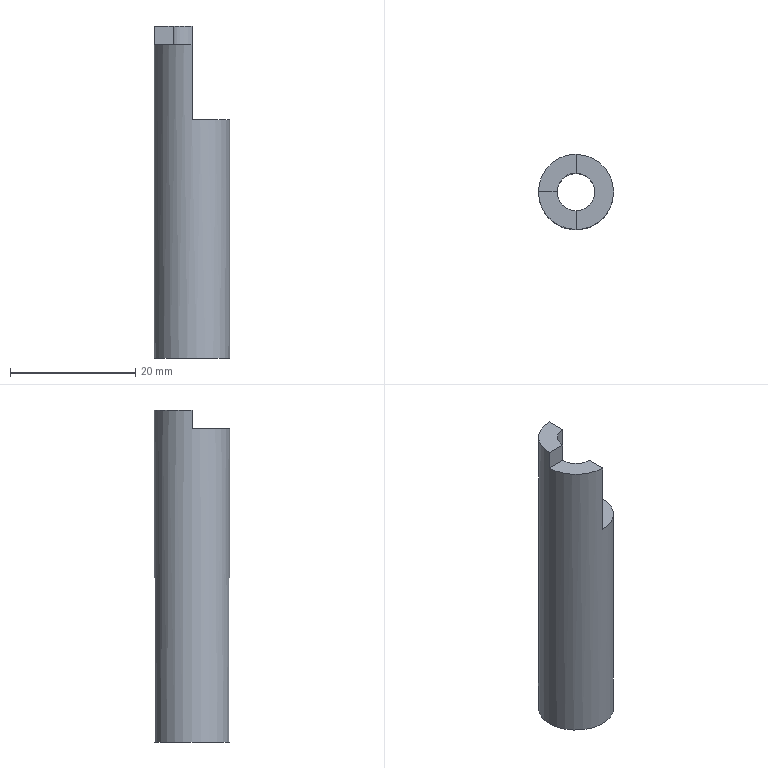Part | NX | features solid 2 | 1 solid | 9 faces | box 12 x 12 x 53 mm | volume 3795 mm3 | plane 7 | cylinder 2 | commonest cylinder face diameters 6.003 x1 12 x1
STEP:
#1=CARTESIAN_POINT('',(3806.088,-895.103,800.716));
#2=VERTEX_POINT('',#1);
#3=CARTESIAN_POINT('',(3806.088,-898.101,800.716));
#4=VERTEX_POINT('',#3);
#5=CARTESIAN_POINT('',(3806.088,-892.101,800.716));
#6=DIRECTION('',(0.,-1.,0.));
#7=VECTOR('',#6,1000.);
#8=LINE('',#5,#7);
#9=EDGE_CURVE('',#2,#4,#8,.T.);
#10=ORIENTED_EDGE('',*,*,#9,.T.);
#11=CARTESIAN_POINT('',(3806.088,-898.101,788.716));
#12=VERTEX_POINT('',#11);
#13=CARTESIAN_POINT('',(3806.088,-898.101,803.716));
#14=DIRECTION('',(0.,0.,-1.));
#15=VECTOR('',#14,1000.);
#16=LINE('',#13,#15);
#17=EDGE_CURVE('',#4,#12,#16,.T.);
#18=ORIENTED_EDGE('',*,*,#17,.T.);
#19=CARTESIAN_POINT('',(3806.088,-895.103,788.716));
#20=VERTEX_POINT('',#19);
#21=CARTESIAN_POINT('',(3806.088,-880.101,788.716));
#22=DIRECTION('',(0.,-1.,0.));
#23=VECTOR('',#22,1000.);
#24=LINE('',#21,#23);
#25=EDGE_CURVE('',#12,#20,#24,.F.);
#26=ORIENTED_EDGE('',*,*,#25,.T.);
#27=CARTESIAN_POINT('',(3806.088,-895.103,803.716));
#28=DIRECTION('',(0.,0.,-1.));
#29=VECTOR('',#28,1000.);
#30=LINE('',#27,#29);
#31=EDGE_CURVE('',#2,#20,#30,.T.);
#32=ORIENTED_EDGE('',*,*,#31,.F.);
#33=EDGE_LOOP('',(#10,#18,#26,#32));
#34=FACE_BOUND('',#33,.T.);
#35=CARTESIAN_POINT('',(3806.088,-880.101,788.716));
#36=DIRECTION('',(-1.,0.,0.));
#37=DIRECTION('',(0.,0.,1.));
#38=AXIS2_PLACEMENT_3D('',#35,#36,#37);
#39=PLANE('',#38);
#40=ADVANCED_FACE('',(#34),#39,.F.);
#41=CARTESIAN_POINT('',(3809.09,-892.101,750.716));
#42=VERTEX_POINT('',#41);
#43=CARTESIAN_POINT('',(3806.088,-892.101,750.716));
#44=DIRECTION('',(0.,0.,1.));
#45=DIRECTION('',(1.,0.,0.));
#46=AXIS2_PLACEMENT_3D('',#43,#44,#45);
#47=CIRCLE('',#46,3.002);
#48=EDGE_CURVE('',#42,#42,#47,.T.);
#49=ORIENTED_EDGE('',*,*,#48,.T.);
#50=EDGE_LOOP('',(#49));
#51=FACE_BOUND('',#50,.T.);
#52=CARTESIAN_POINT('',(3812.088,-892.101,750.716));
#53=VERTEX_POINT('',#52);
#54=CARTESIAN_POINT('',(3806.088,-892.101,750.716));
#55=DIRECTION('',(0.,0.,1.));
#56=DIRECTION('',(1.,0.,0.));
#57=AXIS2_PLACEMENT_3D('',#54,#55,#56);
#58=CIRCLE('',#57,6.);
#59=EDGE_CURVE('',#53,#53,#58,.T.);
#60=ORIENTED_EDGE('',*,*,#59,.F.);
#61=EDGE_LOOP('',(#60));
#62=FACE_BOUND('',#61,.T.);
#63=CARTESIAN_POINT('',(3806.088,-892.101,750.716));
#64=DIRECTION('',(0.,0.,-1.));
#65=DIRECTION('',(-1.,0.,0.));
#66=AXIS2_PLACEMENT_3D('',#63,#64,#65);
#67=PLANE('',#66);
#68=ADVANCED_FACE('',(#51,#62),#67,.T.);
#69=CARTESIAN_POINT('',(3803.087,-892.101,803.716));
#70=VERTEX_POINT('',#69);
#71=CARTESIAN_POINT('',(3800.088,-892.101,803.716));
#72=VERTEX_POINT('',#71);
#73=CARTESIAN_POINT('',(3806.088,-892.101,803.716));
#74=DIRECTION('',(-1.,0.,0.));
#75=VECTOR('',#74,1000.);
#76=LINE('',#73,#75);
#77=EDGE_CURVE('',#70,#72,#76,.T.);
#78=ORIENTED_EDGE('',*,*,#77,.F.);
#79=CARTESIAN_POINT('',(3806.088,-889.1,803.716));
#80=VERTEX_POINT('',#79);
#81=CARTESIAN_POINT('',(3806.088,-892.101,803.716));
#82=DIRECTION('',(0.,0.,-1.));
#83=DIRECTION('',(1.,0.,0.));
#84=AXIS2_PLACEMENT_3D('',#81,#82,#83);
#85=CIRCLE('',#84,3.002);
#86=EDGE_CURVE('',#70,#80,#85,.T.);
#87=ORIENTED_EDGE('',*,*,#86,.T.);
#88=CARTESIAN_POINT('',(3806.088,-886.101,803.716));
#89=VERTEX_POINT('',#88);
#90=CARTESIAN_POINT('',(3806.088,-880.101,803.716));
#91=DIRECTION('',(0.,-1.,0.));
#92=VECTOR('',#91,1000.);
#93=LINE('',#90,#92);
#94=EDGE_CURVE('',#89,#80,#93,.T.);
#95=ORIENTED_EDGE('',*,*,#94,.F.);
#96=CARTESIAN_POINT('',(3806.088,-892.101,803.716));
#97=DIRECTION('',(0.,0.,-1.));
#98=DIRECTION('',(1.,0.,0.));
#99=AXIS2_PLACEMENT_3D('',#96,#97,#98);
#100=CIRCLE('',#99,6.);
#101=EDGE_CURVE('',#72,#89,#100,.T.);
#102=ORIENTED_EDGE('',*,*,#101,.F.);
#103=EDGE_LOOP('',(#78,#87,#95,#102));
#104=FACE_BOUND('',#103,.T.);
#105=CARTESIAN_POINT('',(3806.088,-892.101,803.716));
#106=DIRECTION('',(0.,0.,1.));
#107=DIRECTION('',(1.,0.,0.));
#108=AXIS2_PLACEMENT_3D('',#105,#106,#107);
#109=PLANE('',#108);
#110=ADVANCED_FACE('',(#104),#109,.T.);
#111=CARTESIAN_POINT('',(3800.088,-892.101,800.716));
#112=VERTEX_POINT('',#111);
#113=CARTESIAN_POINT('',(3800.088,-892.101,803.716));
#114=DIRECTION('',(0.,0.,-1.));
#115=VECTOR('',#114,1000.);
#116=LINE('',#113,#115);
#117=EDGE_CURVE('',#72,#112,#116,.T.);
#118=ORIENTED_EDGE('',*,*,#117,.F.);
#119=ORIENTED_EDGE('',*,*,#101,.T.);
#120=CARTESIAN_POINT('',(3806.088,-886.101,788.716));
#121=VERTEX_POINT('',#120);
#122=CARTESIAN_POINT('',(3806.088,-886.101,803.716));
#123=DIRECTION('',(0.,0.,-1.));
#124=VECTOR('',#123,1000.);
#125=LINE('',#122,#124);
#126=EDGE_CURVE('',#121,#89,#125,.F.);
#127=ORIENTED_EDGE('',*,*,#126,.F.);
#128=CARTESIAN_POINT('',(3806.088,-892.101,788.716));
#129=DIRECTION('',(0.,0.,-1.));
#130=DIRECTION('',(-1.,0.,0.));
#131=AXIS2_PLACEMENT_3D('',#128,#129,#130);
#132=CIRCLE('',#131,6.);
#133=EDGE_CURVE('',#12,#121,#132,.F.);
#134=ORIENTED_EDGE('',*,*,#133,.F.);
#135=ORIENTED_EDGE('',*,*,#17,.F.);
#136=CARTESIAN_POINT('',(3806.088,-892.101,800.716));
#137=DIRECTION('',(0.,0.,1.));
#138=DIRECTION('',(1.,0.,0.));
#139=AXIS2_PLACEMENT_3D('',#136,#137,#138);
#140=CIRCLE('',#139,6.);
#141=EDGE_CURVE('',#4,#112,#140,.F.);
#142=ORIENTED_EDGE('',*,*,#141,.T.);
#143=EDGE_LOOP('',(#118,#119,#127,#134,#135,#142));
#144=FACE_BOUND('',#143,.T.);
#145=ORIENTED_EDGE('',*,*,#59,.T.);
#146=EDGE_LOOP('',(#145));
#147=FACE_BOUND('',#146,.T.);
#148=CARTESIAN_POINT('',(3806.088,-892.101,815.716));
#149=DIRECTION('',(0.,0.,-1.));
#150=DIRECTION('',(1.,0.,0.));
#151=AXIS2_PLACEMENT_3D('',#148,#149,#150);
#152=CYLINDRICAL_SURFACE('',#151,6.);
#153=ADVANCED_FACE('',(#144,#147),#152,.T.);
#154=ORIENTED_EDGE('',*,*,#48,.F.);
#155=EDGE_LOOP('',(#154));
#156=FACE_BOUND('',#155,.T.);
#157=ORIENTED_EDGE('',*,*,#86,.F.);
#158=CARTESIAN_POINT('',(3803.087,-892.101,800.716));
#159=VERTEX_POINT('',#158);
#160=CARTESIAN_POINT('',(3803.087,-892.101,803.716));
#161=DIRECTION('',(0.,0.,-1.));
#162=VECTOR('',#161,1000.);
#163=LINE('',#160,#162);
#164=EDGE_CURVE('',#70,#159,#163,.T.);
#165=ORIENTED_EDGE('',*,*,#164,.T.);
#166=CARTESIAN_POINT('',(3806.088,-892.101,800.716));
#167=DIRECTION('',(0.,0.,1.));
#168=DIRECTION('',(1.,0.,0.));
#169=AXIS2_PLACEMENT_3D('',#166,#167,#168);
#170=CIRCLE('',#169,3.002);
#171=EDGE_CURVE('',#2,#159,#170,.F.);
#172=ORIENTED_EDGE('',*,*,#171,.F.);
#173=ORIENTED_EDGE('',*,*,#31,.T.);
#174=CARTESIAN_POINT('',(3806.088,-889.1,788.716));
#175=VERTEX_POINT('',#174);
#176=CARTESIAN_POINT('',(3806.088,-892.101,788.716));
#177=DIRECTION('',(0.,0.,-1.));
#178=DIRECTION('',(-1.,0.,0.));
#179=AXIS2_PLACEMENT_3D('',#176,#177,#178);
#180=CIRCLE('',#179,3.002);
#181=EDGE_CURVE('',#20,#175,#180,.F.);
#182=ORIENTED_EDGE('',*,*,#181,.T.);
#183=CARTESIAN_POINT('',(3806.088,-889.1,803.716));
#184=DIRECTION('',(0.,0.,-1.));
#185=VECTOR('',#184,1000.);
#186=LINE('',#183,#185);
#187=EDGE_CURVE('',#175,#80,#186,.F.);
#188=ORIENTED_EDGE('',*,*,#187,.T.);
#189=EDGE_LOOP('',(#157,#165,#172,#173,#182,#188));
#190=FACE_BOUND('',#189,.T.);
#191=CARTESIAN_POINT('',(3806.088,-892.101,815.716));
#192=DIRECTION('',(0.,0.,-1.));
#193=DIRECTION('',(1.,0.,0.));
#194=AXIS2_PLACEMENT_3D('',#191,#192,#193);
#195=CYLINDRICAL_SURFACE('',#194,3.002);
#196=ADVANCED_FACE('',(#156,#190),#195,.F.);
#197=ORIENTED_EDGE('',*,*,#126,.T.);
#198=ORIENTED_EDGE('',*,*,#94,.T.);
#199=ORIENTED_EDGE('',*,*,#187,.F.);
#200=CARTESIAN_POINT('',(3806.088,-880.101,788.716));
#201=DIRECTION('',(0.,-1.,0.));
#202=VECTOR('',#201,1000.);
#203=LINE('',#200,#202);
#204=EDGE_CURVE('',#175,#121,#203,.F.);
#205=ORIENTED_EDGE('',*,*,#204,.T.);
#206=EDGE_LOOP('',(#197,#198,#199,#205));
#207=FACE_BOUND('',#206,.T.);
#208=CARTESIAN_POINT('',(3806.088,-880.101,788.716));
#209=DIRECTION('',(-1.,0.,0.));
#210=DIRECTION('',(0.,0.,1.));
#211=AXIS2_PLACEMENT_3D('',#208,#209,#210);
#212=PLANE('',#211);
#213=ADVANCED_FACE('',(#207),#212,.F.);
#214=ORIENTED_EDGE('',*,*,#133,.T.);
#215=ORIENTED_EDGE('',*,*,#204,.F.);
#216=ORIENTED_EDGE('',*,*,#181,.F.);
#217=ORIENTED_EDGE('',*,*,#25,.F.);
#218=EDGE_LOOP('',(#214,#215,#216,#217));
#219=FACE_BOUND('',#218,.T.);
#220=CARTESIAN_POINT('',(146.,0.,788.716));
#221=DIRECTION('',(0.,0.,-1.));
#222=DIRECTION('',(-1.,0.,0.));
#223=AXIS2_PLACEMENT_3D('',#220,#221,#222);
#224=PLANE('',#223);
#225=ADVANCED_FACE('',(#219),#224,.F.);
#226=ORIENTED_EDGE('',*,*,#117,.T.);
#227=CARTESIAN_POINT('',(3806.088,-892.101,800.716));
#228=DIRECTION('',(-1.,0.,0.));
#229=VECTOR('',#228,1000.);
#230=LINE('',#227,#229);
#231=EDGE_CURVE('',#112,#159,#230,.F.);
#232=ORIENTED_EDGE('',*,*,#231,.T.);
#233=ORIENTED_EDGE('',*,*,#164,.F.);
#234=ORIENTED_EDGE('',*,*,#77,.T.);
#235=EDGE_LOOP('',(#226,#232,#233,#234));
#236=FACE_BOUND('',#235,.T.);
#237=CARTESIAN_POINT('',(3806.088,-892.101,800.716));
#238=DIRECTION('',(0.,1.,0.));
#239=DIRECTION('',(0.,0.,1.));
#240=AXIS2_PLACEMENT_3D('',#237,#238,#239);
#241=PLANE('',#240);
#242=ADVANCED_FACE('',(#236),#241,.F.);
#243=ORIENTED_EDGE('',*,*,#9,.F.);
#244=ORIENTED_EDGE('',*,*,#171,.T.);
#245=ORIENTED_EDGE('',*,*,#231,.F.);
#246=ORIENTED_EDGE('',*,*,#141,.F.);
#247=EDGE_LOOP('',(#243,#244,#245,#246));
#248=FACE_BOUND('',#247,.T.);
#249=CARTESIAN_POINT('',(146.,0.,800.716));
#250=DIRECTION('',(0.,0.,1.));
#251=DIRECTION('',(1.,0.,0.));
#252=AXIS2_PLACEMENT_3D('',#249,#250,#251);
#253=PLANE('',#252);
#254=ADVANCED_FACE('',(#248),#253,.T.);
#255=CLOSED_SHELL('',(#40,#68,#110,#153,#196,#213,#225,#242,#254));
#256=MANIFOLD_SOLID_BREP('',#255);
#257=(LENGTH_UNIT()NAMED_UNIT(*)SI_UNIT(.MILLI.,.METRE.));
#258=UNCERTAINTY_MEASURE_WITH_UNIT(LENGTH_MEASURE(0.00001),#257,'','');
#259=(NAMED_UNIT(*)PLANE_ANGLE_UNIT()SI_UNIT($,.RADIAN.));
#260=(NAMED_UNIT(*)SI_UNIT($,.STERADIAN.)SOLID_ANGLE_UNIT());
#261=(GEOMETRIC_REPRESENTATION_CONTEXT(3)GLOBAL_UNCERTAINTY_ASSIGNED_CONTEXT((#258))GLOBAL_UNIT_ASSIGNED_CONTEXT((#257,#259,#260))REPRESENTATION_CONTEXT('',''));
#262=ADVANCED_BREP_SHAPE_REPRESENTATION('',(#256),#261);